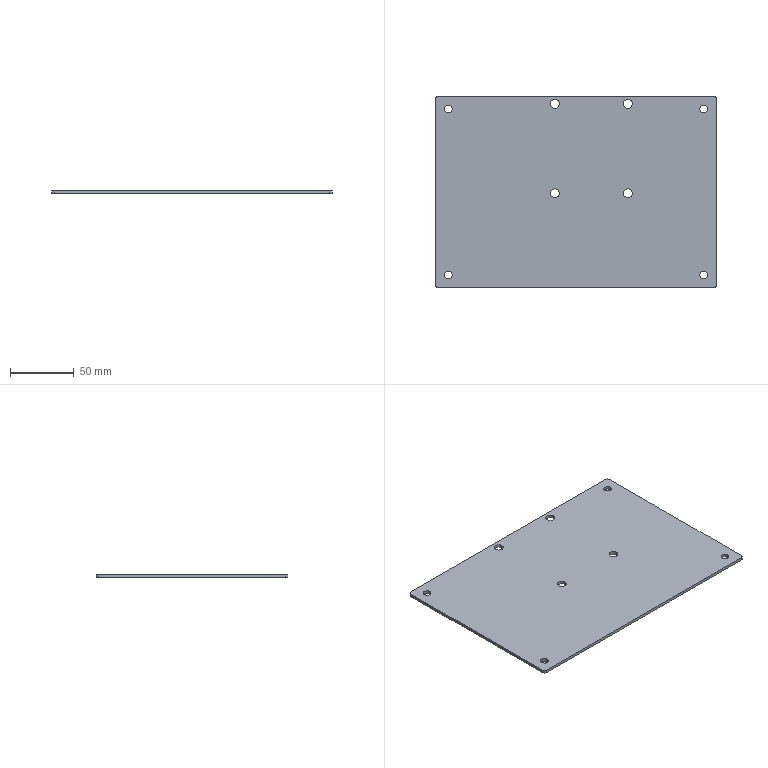Part | STEP file | Second M80U005006A Air System BKT Default | 1 solid | 26 faces | box 220 x 150 x 2.3 mm | volume 75278 mm3 | cylinder 20 | plane 6 | commonest cylinder face diameters 6 x8 7 x8 4 x4
STEP:
#1=CARTESIAN_POINT('',(-20.,69.,0.));
#2=VERTEX_POINT('',#1);
#3=CARTESIAN_POINT('',(-13.,69.,0.));
#4=VERTEX_POINT('',#3);
#5=CARTESIAN_POINT('',(-16.5,69.,0.));
#6=DIRECTION('',(0.,0.,1.));
#7=DIRECTION('',(1.,0.,0.));
#8=AXIS2_PLACEMENT_3D('',#5,#6,#7);
#9=CIRCLE('',#8,3.5);
#10=EDGE_CURVE('',#2,#4,#9,.T.);
#11=ORIENTED_EDGE('',*,*,#10,.F.);
#12=CARTESIAN_POINT('',(-20.,69.,2.3));
#13=VERTEX_POINT('',#12);
#14=CARTESIAN_POINT('',(-20.,69.,2.3));
#15=DIRECTION('',(0.,0.,1.));
#16=VECTOR('',#15,1000.);
#17=LINE('',#14,#16);
#18=EDGE_CURVE('',#2,#13,#17,.T.);
#19=ORIENTED_EDGE('',*,*,#18,.T.);
#20=CARTESIAN_POINT('',(-13.,69.,2.3));
#21=VERTEX_POINT('',#20);
#22=CARTESIAN_POINT('',(-16.5,69.,2.3));
#23=DIRECTION('',(0.,0.,1.));
#24=DIRECTION('',(1.,0.,0.));
#25=AXIS2_PLACEMENT_3D('',#22,#23,#24);
#26=CIRCLE('',#25,3.5);
#27=EDGE_CURVE('',#13,#21,#26,.T.);
#28=ORIENTED_EDGE('',*,*,#27,.T.);
#29=CARTESIAN_POINT('',(-13.,69.,2.3));
#30=DIRECTION('',(0.,0.,1.));
#31=VECTOR('',#30,1000.);
#32=LINE('',#29,#31);
#33=EDGE_CURVE('',#4,#21,#32,.T.);
#34=ORIENTED_EDGE('',*,*,#33,.F.);
#35=EDGE_LOOP('',(#11,#19,#28,#34));
#36=FACE_OUTER_BOUND('',#35,.T.);
#37=CARTESIAN_POINT('',(-16.5,69.,2.3));
#38=DIRECTION('',(0.,0.,1.));
#39=DIRECTION('',(1.,0.,0.));
#40=AXIS2_PLACEMENT_3D('',#37,#38,#39);
#41=CYLINDRICAL_SURFACE('',#40,3.5);
#42=ADVANCED_FACE('',(#36),#41,.F.);
#43=CARTESIAN_POINT('',(37.,69.,0.));
#44=VERTEX_POINT('',#43);
#45=CARTESIAN_POINT('',(44.,69.,0.));
#46=VERTEX_POINT('',#45);
#47=CARTESIAN_POINT('',(40.5,69.,0.));
#48=DIRECTION('',(0.,0.,1.));
#49=DIRECTION('',(1.,0.,0.));
#50=AXIS2_PLACEMENT_3D('',#47,#48,#49);
#51=CIRCLE('',#50,3.5);
#52=EDGE_CURVE('',#44,#46,#51,.T.);
#53=ORIENTED_EDGE('',*,*,#52,.F.);
#54=CARTESIAN_POINT('',(37.,69.,2.3));
#55=VERTEX_POINT('',#54);
#56=CARTESIAN_POINT('',(37.,69.,2.3));
#57=DIRECTION('',(0.,0.,1.));
#58=VECTOR('',#57,1000.);
#59=LINE('',#56,#58);
#60=EDGE_CURVE('',#44,#55,#59,.T.);
#61=ORIENTED_EDGE('',*,*,#60,.T.);
#62=CARTESIAN_POINT('',(44.,69.,2.3));
#63=VERTEX_POINT('',#62);
#64=CARTESIAN_POINT('',(40.5,69.,2.3));
#65=DIRECTION('',(0.,0.,1.));
#66=DIRECTION('',(1.,0.,0.));
#67=AXIS2_PLACEMENT_3D('',#64,#65,#66);
#68=CIRCLE('',#67,3.5);
#69=EDGE_CURVE('',#55,#63,#68,.T.);
#70=ORIENTED_EDGE('',*,*,#69,.T.);
#71=CARTESIAN_POINT('',(44.,69.,2.3));
#72=DIRECTION('',(0.,0.,1.));
#73=VECTOR('',#72,1000.);
#74=LINE('',#71,#73);
#75=EDGE_CURVE('',#46,#63,#74,.T.);
#76=ORIENTED_EDGE('',*,*,#75,.F.);
#77=EDGE_LOOP('',(#53,#61,#70,#76));
#78=FACE_OUTER_BOUND('',#77,.T.);
#79=CARTESIAN_POINT('',(40.5,69.,2.3));
#80=DIRECTION('',(0.,0.,1.));
#81=DIRECTION('',(1.,0.,0.));
#82=AXIS2_PLACEMENT_3D('',#79,#80,#81);
#83=CYLINDRICAL_SURFACE('',#82,3.5);
#84=ADVANCED_FACE('',(#78),#83,.F.);
#85=CARTESIAN_POINT('',(37.,-1.,0.));
#86=VERTEX_POINT('',#85);
#87=CARTESIAN_POINT('',(44.,-1.,0.));
#88=VERTEX_POINT('',#87);
#89=CARTESIAN_POINT('',(40.5,-1.,0.));
#90=DIRECTION('',(0.,0.,1.));
#91=DIRECTION('',(1.,0.,0.));
#92=AXIS2_PLACEMENT_3D('',#89,#90,#91);
#93=CIRCLE('',#92,3.5);
#94=EDGE_CURVE('',#86,#88,#93,.T.);
#95=ORIENTED_EDGE('',*,*,#94,.F.);
#96=CARTESIAN_POINT('',(37.,-1.,2.3));
#97=VERTEX_POINT('',#96);
#98=CARTESIAN_POINT('',(37.,-1.,2.3));
#99=DIRECTION('',(0.,0.,1.));
#100=VECTOR('',#99,1000.);
#101=LINE('',#98,#100);
#102=EDGE_CURVE('',#86,#97,#101,.T.);
#103=ORIENTED_EDGE('',*,*,#102,.T.);
#104=CARTESIAN_POINT('',(44.,-1.,2.3));
#105=VERTEX_POINT('',#104);
#106=CARTESIAN_POINT('',(40.5,-1.,2.3));
#107=DIRECTION('',(0.,0.,1.));
#108=DIRECTION('',(1.,0.,0.));
#109=AXIS2_PLACEMENT_3D('',#106,#107,#108);
#110=CIRCLE('',#109,3.5);
#111=EDGE_CURVE('',#97,#105,#110,.T.);
#112=ORIENTED_EDGE('',*,*,#111,.T.);
#113=CARTESIAN_POINT('',(44.,-1.,2.3));
#114=DIRECTION('',(0.,0.,1.));
#115=VECTOR('',#114,1000.);
#116=LINE('',#113,#115);
#117=EDGE_CURVE('',#88,#105,#116,.T.);
#118=ORIENTED_EDGE('',*,*,#117,.F.);
#119=EDGE_LOOP('',(#95,#103,#112,#118));
#120=FACE_OUTER_BOUND('',#119,.T.);
#121=CARTESIAN_POINT('',(40.5,-1.,2.3));
#122=DIRECTION('',(0.,0.,1.));
#123=DIRECTION('',(1.,0.,0.));
#124=AXIS2_PLACEMENT_3D('',#121,#122,#123);
#125=CYLINDRICAL_SURFACE('',#124,3.5);
#126=ADVANCED_FACE('',(#120),#125,.F.);
#127=CARTESIAN_POINT('',(-20.,-1.,0.));
#128=VERTEX_POINT('',#127);
#129=CARTESIAN_POINT('',(-13.,-1.,0.));
#130=VERTEX_POINT('',#129);
#131=CARTESIAN_POINT('',(-16.5,-1.,0.));
#132=DIRECTION('',(0.,0.,1.));
#133=DIRECTION('',(1.,0.,0.));
#134=AXIS2_PLACEMENT_3D('',#131,#132,#133);
#135=CIRCLE('',#134,3.5);
#136=EDGE_CURVE('',#128,#130,#135,.T.);
#137=ORIENTED_EDGE('',*,*,#136,.F.);
#138=CARTESIAN_POINT('',(-20.,-1.,2.3));
#139=VERTEX_POINT('',#138);
#140=CARTESIAN_POINT('',(-20.,-1.,2.3));
#141=DIRECTION('',(0.,0.,1.));
#142=VECTOR('',#141,1000.);
#143=LINE('',#140,#142);
#144=EDGE_CURVE('',#128,#139,#143,.T.);
#145=ORIENTED_EDGE('',*,*,#144,.T.);
#146=CARTESIAN_POINT('',(-13.,-1.,2.3));
#147=VERTEX_POINT('',#146);
#148=CARTESIAN_POINT('',(-16.5,-1.,2.3));
#149=DIRECTION('',(0.,0.,1.));
#150=DIRECTION('',(1.,0.,0.));
#151=AXIS2_PLACEMENT_3D('',#148,#149,#150);
#152=CIRCLE('',#151,3.5);
#153=EDGE_CURVE('',#139,#147,#152,.T.);
#154=ORIENTED_EDGE('',*,*,#153,.T.);
#155=CARTESIAN_POINT('',(-13.,-1.,2.3));
#156=DIRECTION('',(0.,0.,1.));
#157=VECTOR('',#156,1000.);
#158=LINE('',#155,#157);
#159=EDGE_CURVE('',#130,#147,#158,.T.);
#160=ORIENTED_EDGE('',*,*,#159,.F.);
#161=EDGE_LOOP('',(#137,#145,#154,#160));
#162=FACE_OUTER_BOUND('',#161,.T.);
#163=CARTESIAN_POINT('',(-16.5,-1.,2.3));
#164=DIRECTION('',(0.,0.,1.));
#165=DIRECTION('',(1.,0.,0.));
#166=AXIS2_PLACEMENT_3D('',#163,#164,#165);
#167=CYLINDRICAL_SURFACE('',#166,3.5);
#168=ADVANCED_FACE('',(#162),#167,.F.);
#169=CARTESIAN_POINT('',(-103.,65.,0.));
#170=VERTEX_POINT('',#169);
#171=CARTESIAN_POINT('',(-97.,65.,0.));
#172=VERTEX_POINT('',#171);
#173=CARTESIAN_POINT('',(-100.,65.,0.));
#174=DIRECTION('',(0.,0.,1.));
#175=DIRECTION('',(1.,0.,0.));
#176=AXIS2_PLACEMENT_3D('',#173,#174,#175);
#177=CIRCLE('',#176,3.);
#178=EDGE_CURVE('',#170,#172,#177,.T.);
#179=ORIENTED_EDGE('',*,*,#178,.F.);
#180=CARTESIAN_POINT('',(-103.,65.,2.3));
#181=VERTEX_POINT('',#180);
#182=CARTESIAN_POINT('',(-103.,65.,2.3));
#183=DIRECTION('',(0.,0.,1.));
#184=VECTOR('',#183,1000.);
#185=LINE('',#182,#184);
#186=EDGE_CURVE('',#170,#181,#185,.T.);
#187=ORIENTED_EDGE('',*,*,#186,.T.);
#188=CARTESIAN_POINT('',(-97.,65.,2.3));
#189=VERTEX_POINT('',#188);
#190=CARTESIAN_POINT('',(-100.,65.,2.3));
#191=DIRECTION('',(0.,0.,1.));
#192=DIRECTION('',(1.,0.,0.));
#193=AXIS2_PLACEMENT_3D('',#190,#191,#192);
#194=CIRCLE('',#193,3.);
#195=EDGE_CURVE('',#181,#189,#194,.T.);
#196=ORIENTED_EDGE('',*,*,#195,.T.);
#197=CARTESIAN_POINT('',(-97.,65.,2.3));
#198=DIRECTION('',(0.,0.,1.));
#199=VECTOR('',#198,1000.);
#200=LINE('',#197,#199);
#201=EDGE_CURVE('',#172,#189,#200,.T.);
#202=ORIENTED_EDGE('',*,*,#201,.F.);
#203=EDGE_LOOP('',(#179,#187,#196,#202));
#204=FACE_OUTER_BOUND('',#203,.T.);
#205=CARTESIAN_POINT('',(-100.,65.,2.3));
#206=DIRECTION('',(0.,0.,1.));
#207=DIRECTION('',(1.,0.,0.));
#208=AXIS2_PLACEMENT_3D('',#205,#206,#207);
#209=CYLINDRICAL_SURFACE('',#208,3.);
#210=ADVANCED_FACE('',(#204),#209,.F.);
#211=CARTESIAN_POINT('',(-103.,-65.,0.));
#212=VERTEX_POINT('',#211);
#213=CARTESIAN_POINT('',(-97.,-65.,0.));
#214=VERTEX_POINT('',#213);
#215=CARTESIAN_POINT('',(-100.,-65.,0.));
#216=DIRECTION('',(0.,0.,1.));
#217=DIRECTION('',(1.,0.,0.));
#218=AXIS2_PLACEMENT_3D('',#215,#216,#217);
#219=CIRCLE('',#218,3.);
#220=EDGE_CURVE('',#212,#214,#219,.T.);
#221=ORIENTED_EDGE('',*,*,#220,.F.);
#222=CARTESIAN_POINT('',(-103.,-65.,2.3));
#223=VERTEX_POINT('',#222);
#224=CARTESIAN_POINT('',(-103.,-65.,2.3));
#225=DIRECTION('',(0.,0.,1.));
#226=VECTOR('',#225,1000.);
#227=LINE('',#224,#226);
#228=EDGE_CURVE('',#212,#223,#227,.T.);
#229=ORIENTED_EDGE('',*,*,#228,.T.);
#230=CARTESIAN_POINT('',(-97.,-65.,2.3));
#231=VERTEX_POINT('',#230);
#232=CARTESIAN_POINT('',(-100.,-65.,2.3));
#233=DIRECTION('',(0.,0.,1.));
#234=DIRECTION('',(1.,0.,0.));
#235=AXIS2_PLACEMENT_3D('',#232,#233,#234);
#236=CIRCLE('',#235,3.);
#237=EDGE_CURVE('',#223,#231,#236,.T.);
#238=ORIENTED_EDGE('',*,*,#237,.T.);
#239=CARTESIAN_POINT('',(-97.,-65.,2.3));
#240=DIRECTION('',(0.,0.,1.));
#241=VECTOR('',#240,1000.);
#242=LINE('',#239,#241);
#243=EDGE_CURVE('',#214,#231,#242,.T.);
#244=ORIENTED_EDGE('',*,*,#243,.F.);
#245=EDGE_LOOP('',(#221,#229,#238,#244));
#246=FACE_OUTER_BOUND('',#245,.T.);
#247=CARTESIAN_POINT('',(-100.,-65.,2.3));
#248=DIRECTION('',(0.,0.,1.));
#249=DIRECTION('',(1.,0.,0.));
#250=AXIS2_PLACEMENT_3D('',#247,#248,#249);
#251=CYLINDRICAL_SURFACE('',#250,3.);
#252=ADVANCED_FACE('',(#246),#251,.F.);
#253=CARTESIAN_POINT('',(97.,-65.,0.));
#254=VERTEX_POINT('',#253);
#255=CARTESIAN_POINT('',(103.,-65.,0.));
#256=VERTEX_POINT('',#255);
#257=CARTESIAN_POINT('',(100.,-65.,0.));
#258=DIRECTION('',(0.,0.,1.));
#259=DIRECTION('',(1.,0.,0.));
#260=AXIS2_PLACEMENT_3D('',#257,#258,#259);
#261=CIRCLE('',#260,3.);
#262=EDGE_CURVE('',#254,#256,#261,.T.);
#263=ORIENTED_EDGE('',*,*,#262,.F.);
#264=CARTESIAN_POINT('',(97.,-65.,2.3));
#265=VERTEX_POINT('',#264);
#266=CARTESIAN_POINT('',(97.,-65.,2.3));
#267=DIRECTION('',(0.,0.,1.));
#268=VECTOR('',#267,1000.);
#269=LINE('',#266,#268);
#270=EDGE_CURVE('',#254,#265,#269,.T.);
#271=ORIENTED_EDGE('',*,*,#270,.T.);
#272=CARTESIAN_POINT('',(103.,-65.,2.3));
#273=VERTEX_POINT('',#272);
#274=CARTESIAN_POINT('',(100.,-65.,2.3));
#275=DIRECTION('',(0.,0.,1.));
#276=DIRECTION('',(1.,0.,0.));
#277=AXIS2_PLACEMENT_3D('',#274,#275,#276);
#278=CIRCLE('',#277,3.);
#279=EDGE_CURVE('',#265,#273,#278,.T.);
#280=ORIENTED_EDGE('',*,*,#279,.T.);
#281=CARTESIAN_POINT('',(103.,-65.,2.3));
#282=DIRECTION('',(0.,0.,1.));
#283=VECTOR('',#282,1000.);
#284=LINE('',#281,#283);
#285=EDGE_CURVE('',#256,#273,#284,.T.);
#286=ORIENTED_EDGE('',*,*,#285,.F.);
#287=EDGE_LOOP('',(#263,#271,#280,#286));
#288=FACE_OUTER_BOUND('',#287,.T.);
#289=CARTESIAN_POINT('',(100.,-65.,2.3));
#290=DIRECTION('',(0.,0.,1.));
#291=DIRECTION('',(1.,0.,0.));
#292=AXIS2_PLACEMENT_3D('',#289,#290,#291);
#293=CYLINDRICAL_SURFACE('',#292,3.);
#294=ADVANCED_FACE('',(#288),#293,.F.);
#295=CARTESIAN_POINT('',(97.,65.,0.));
#296=VERTEX_POINT('',#295);
#297=CARTESIAN_POINT('',(103.,65.,0.));
#298=VERTEX_POINT('',#297);
#299=CARTESIAN_POINT('',(100.,65.,0.));
#300=DIRECTION('',(0.,0.,1.));
#301=DIRECTION('',(1.,0.,0.));
#302=AXIS2_PLACEMENT_3D('',#299,#300,#301);
#303=CIRCLE('',#302,3.);
#304=EDGE_CURVE('',#296,#298,#303,.T.);
#305=ORIENTED_EDGE('',*,*,#304,.F.);
#306=CARTESIAN_POINT('',(97.,65.,2.3));
#307=VERTEX_POINT('',#306);
#308=CARTESIAN_POINT('',(97.,65.,2.3));
#309=DIRECTION('',(0.,0.,1.));
#310=VECTOR('',#309,1000.);
#311=LINE('',#308,#310);
#312=EDGE_CURVE('',#296,#307,#311,.T.);
#313=ORIENTED_EDGE('',*,*,#312,.T.);
#314=CARTESIAN_POINT('',(103.,65.,2.3));
#315=VERTEX_POINT('',#314);
#316=CARTESIAN_POINT('',(100.,65.,2.3));
#317=DIRECTION('',(0.,0.,1.));
#318=DIRECTION('',(1.,0.,0.));
#319=AXIS2_PLACEMENT_3D('',#316,#317,#318);
#320=CIRCLE('',#319,3.);
#321=EDGE_CURVE('',#307,#315,#320,.T.);
#322=ORIENTED_EDGE('',*,*,#321,.T.);
#323=CARTESIAN_POINT('',(103.,65.,2.3));
#324=DIRECTION('',(0.,0.,1.));
#325=VECTOR('',#324,1000.);
#326=LINE('',#323,#325);
#327=EDGE_CURVE('',#298,#315,#326,.T.);
#328=ORIENTED_EDGE('',*,*,#327,.F.);
#329=EDGE_LOOP('',(#305,#313,#322,#328));
#330=FACE_OUTER_BOUND('',#329,.T.);
#331=CARTESIAN_POINT('',(100.,65.,2.3));
#332=DIRECTION('',(0.,0.,1.));
#333=DIRECTION('',(1.,0.,0.));
#334=AXIS2_PLACEMENT_3D('',#331,#332,#333);
#335=CYLINDRICAL_SURFACE('',#334,3.);
#336=ADVANCED_FACE('',(#330),#335,.F.);
#337=CARTESIAN_POINT('',(-110.,73.,0.));
#338=VERTEX_POINT('',#337);
#339=CARTESIAN_POINT('',(-110.,-73.,0.));
#340=VERTEX_POINT('',#339);
#341=CARTESIAN_POINT('',(-110.,-75.,0.));
#342=DIRECTION('',(0.,-1.,0.));
#343=VECTOR('',#342,1000.);
#344=LINE('',#341,#343);
#345=EDGE_CURVE('',#338,#340,#344,.T.);
#346=ORIENTED_EDGE('',*,*,#345,.T.);
#347=CARTESIAN_POINT('',(-110.,-73.,2.3));
#348=VERTEX_POINT('',#347);
#349=CARTESIAN_POINT('',(-110.,-73.,2.3));
#350=DIRECTION('',(0.,0.,1.));
#351=VECTOR('',#350,1000.);
#352=LINE('',#349,#351);
#353=EDGE_CURVE('',#340,#348,#352,.T.);
#354=ORIENTED_EDGE('',*,*,#353,.T.);
#355=CARTESIAN_POINT('',(-110.,73.,2.3));
#356=VERTEX_POINT('',#355);
#357=CARTESIAN_POINT('',(-110.,-75.,2.3));
#358=DIRECTION('',(0.,-1.,0.));
#359=VECTOR('',#358,1000.);
#360=LINE('',#357,#359);
#361=EDGE_CURVE('',#356,#348,#360,.T.);
#362=ORIENTED_EDGE('',*,*,#361,.F.);
#363=CARTESIAN_POINT('',(-110.,73.,2.3));
#364=DIRECTION('',(0.,0.,-1.));
#365=VECTOR('',#364,1000.);
#366=LINE('',#363,#365);
#367=EDGE_CURVE('',#356,#338,#366,.T.);
#368=ORIENTED_EDGE('',*,*,#367,.T.);
#369=EDGE_LOOP('',(#346,#354,#362,#368));
#370=FACE_OUTER_BOUND('',#369,.T.);
#371=CARTESIAN_POINT('',(-110.,-75.,2.3));
#372=DIRECTION('',(1.,0.,0.));
#373=DIRECTION('',(0.,0.,-1.));
#374=AXIS2_PLACEMENT_3D('',#371,#372,#373);
#375=PLANE('',#374);
#376=ADVANCED_FACE('',(#370),#375,.F.);
#377=CARTESIAN_POINT('',(-108.,-75.,0.));
#378=VERTEX_POINT('',#377);
#379=CARTESIAN_POINT('',(108.,-75.,0.));
#380=VERTEX_POINT('',#379);
#381=CARTESIAN_POINT('',(110.,-75.,0.));
#382=DIRECTION('',(1.,0.,0.));
#383=VECTOR('',#382,1000.);
#384=LINE('',#381,#383);
#385=EDGE_CURVE('',#378,#380,#384,.T.);
#386=ORIENTED_EDGE('',*,*,#385,.T.);
#387=CARTESIAN_POINT('',(108.,-75.,2.3));
#388=VERTEX_POINT('',#387);
#389=CARTESIAN_POINT('',(108.,-75.,2.3));
#390=DIRECTION('',(0.,0.,1.));
#391=VECTOR('',#390,1000.);
#392=LINE('',#389,#391);
#393=EDGE_CURVE('',#380,#388,#392,.T.);
#394=ORIENTED_EDGE('',*,*,#393,.T.);
#395=CARTESIAN_POINT('',(-108.,-75.,2.3));
#396=VERTEX_POINT('',#395);
#397=CARTESIAN_POINT('',(110.,-75.,2.3));
#398=DIRECTION('',(1.,0.,0.));
#399=VECTOR('',#398,1000.);
#400=LINE('',#397,#399);
#401=EDGE_CURVE('',#396,#388,#400,.T.);
#402=ORIENTED_EDGE('',*,*,#401,.F.);
#403=CARTESIAN_POINT('',(-108.,-75.,2.3));
#404=DIRECTION('',(0.,0.,-1.));
#405=VECTOR('',#404,1000.);
#406=LINE('',#403,#405);
#407=EDGE_CURVE('',#396,#378,#406,.T.);
#408=ORIENTED_EDGE('',*,*,#407,.T.);
#409=EDGE_LOOP('',(#386,#394,#402,#408));
#410=FACE_OUTER_BOUND('',#409,.T.);
#411=CARTESIAN_POINT('',(110.,-75.,2.3));
#412=DIRECTION('',(0.,1.,0.));
#413=DIRECTION('',(-1.,0.,0.));
#414=AXIS2_PLACEMENT_3D('',#411,#412,#413);
#415=PLANE('',#414);
#416=ADVANCED_FACE('',(#410),#415,.F.);
#417=CARTESIAN_POINT('',(110.,-73.,0.));
#418=VERTEX_POINT('',#417);
#419=CARTESIAN_POINT('',(110.,73.,0.));
#420=VERTEX_POINT('',#419);
#421=CARTESIAN_POINT('',(110.,-75.,0.));
#422=DIRECTION('',(0.,1.,0.));
#423=VECTOR('',#422,1000.);
#424=LINE('',#421,#423);
#425=EDGE_CURVE('',#418,#420,#424,.T.);
#426=ORIENTED_EDGE('',*,*,#425,.T.);
#427=CARTESIAN_POINT('',(110.,73.,2.3));
#428=VERTEX_POINT('',#427);
#429=CARTESIAN_POINT('',(110.,73.,2.3));
#430=DIRECTION('',(0.,0.,1.));
#431=VECTOR('',#430,1000.);
#432=LINE('',#429,#431);
#433=EDGE_CURVE('',#420,#428,#432,.T.);
#434=ORIENTED_EDGE('',*,*,#433,.T.);
#435=CARTESIAN_POINT('',(110.,-73.,2.3));
#436=VERTEX_POINT('',#435);
#437=CARTESIAN_POINT('',(110.,-75.,2.3));
#438=DIRECTION('',(0.,1.,0.));
#439=VECTOR('',#438,1000.);
#440=LINE('',#437,#439);
#441=EDGE_CURVE('',#436,#428,#440,.T.);
#442=ORIENTED_EDGE('',*,*,#441,.F.);
#443=CARTESIAN_POINT('',(110.,-73.,2.3));
#444=DIRECTION('',(0.,0.,-1.));
#445=VECTOR('',#444,1000.);
#446=LINE('',#443,#445);
#447=EDGE_CURVE('',#436,#418,#446,.T.);
#448=ORIENTED_EDGE('',*,*,#447,.T.);
#449=EDGE_LOOP('',(#426,#434,#442,#448));
#450=FACE_OUTER_BOUND('',#449,.T.);
#451=CARTESIAN_POINT('',(110.,-75.,2.3));
#452=DIRECTION('',(-1.,0.,0.));
#453=DIRECTION('',(0.,0.,1.));
#454=AXIS2_PLACEMENT_3D('',#451,#452,#453);
#455=PLANE('',#454);
#456=ADVANCED_FACE('',(#450),#455,.F.);
#457=CARTESIAN_POINT('',(108.,75.,2.3));
#458=VERTEX_POINT('',#457);
#459=CARTESIAN_POINT('',(-108.,75.,2.3));
#460=VERTEX_POINT('',#459);
#461=CARTESIAN_POINT('',(110.,75.,2.3));
#462=DIRECTION('',(-1.,0.,0.));
#463=VECTOR('',#462,1000.);
#464=LINE('',#461,#463);
#465=EDGE_CURVE('',#458,#460,#464,.T.);
#466=ORIENTED_EDGE('',*,*,#465,.F.);
#467=CARTESIAN_POINT('',(108.,75.,0.));
#468=VERTEX_POINT('',#467);
#469=CARTESIAN_POINT('',(108.,75.,2.3));
#470=DIRECTION('',(0.,0.,-1.));
#471=VECTOR('',#470,1000.);
#472=LINE('',#469,#471);
#473=EDGE_CURVE('',#458,#468,#472,.T.);
#474=ORIENTED_EDGE('',*,*,#473,.T.);
#475=CARTESIAN_POINT('',(-108.,75.,0.));
#476=VERTEX_POINT('',#475);
#477=CARTESIAN_POINT('',(110.,75.,0.));
#478=DIRECTION('',(-1.,0.,0.));
#479=VECTOR('',#478,1000.);
#480=LINE('',#477,#479);
#481=EDGE_CURVE('',#468,#476,#480,.T.);
#482=ORIENTED_EDGE('',*,*,#481,.T.);
#483=CARTESIAN_POINT('',(-108.,75.,2.3));
#484=DIRECTION('',(0.,0.,1.));
#485=VECTOR('',#484,1000.);
#486=LINE('',#483,#485);
#487=EDGE_CURVE('',#476,#460,#486,.T.);
#488=ORIENTED_EDGE('',*,*,#487,.T.);
#489=EDGE_LOOP('',(#466,#474,#482,#488));
#490=FACE_OUTER_BOUND('',#489,.T.);
#491=CARTESIAN_POINT('',(110.,75.,2.3));
#492=DIRECTION('',(0.,-1.,0.));
#493=DIRECTION('',(1.,0.,0.));
#494=AXIS2_PLACEMENT_3D('',#491,#492,#493);
#495=PLANE('',#494);
#496=ADVANCED_FACE('',(#490),#495,.F.);
#497=CARTESIAN_POINT('',(-16.5,69.,2.3));
#498=DIRECTION('',(0.,0.,1.));
#499=DIRECTION('',(1.,0.,0.));
#500=AXIS2_PLACEMENT_3D('',#497,#498,#499);
#501=CIRCLE('',#500,3.5);
#502=EDGE_CURVE('',#21,#13,#501,.T.);
#503=ORIENTED_EDGE('',*,*,#502,.F.);
#504=ORIENTED_EDGE('',*,*,#27,.F.);
#505=EDGE_LOOP('',(#503,#504));
#506=FACE_BOUND('',#505,.T.);
#507=CARTESIAN_POINT('',(40.5,69.,2.3));
#508=DIRECTION('',(0.,0.,1.));
#509=DIRECTION('',(1.,0.,0.));
#510=AXIS2_PLACEMENT_3D('',#507,#508,#509);
#511=CIRCLE('',#510,3.5);
#512=EDGE_CURVE('',#63,#55,#511,.T.);
#513=ORIENTED_EDGE('',*,*,#512,.F.);
#514=ORIENTED_EDGE('',*,*,#69,.F.);
#515=EDGE_LOOP('',(#513,#514));
#516=FACE_BOUND('',#515,.T.);
#517=CARTESIAN_POINT('',(40.5,-1.,2.3));
#518=DIRECTION('',(0.,0.,1.));
#519=DIRECTION('',(1.,0.,0.));
#520=AXIS2_PLACEMENT_3D('',#517,#518,#519);
#521=CIRCLE('',#520,3.5);
#522=EDGE_CURVE('',#105,#97,#521,.T.);
#523=ORIENTED_EDGE('',*,*,#522,.F.);
#524=ORIENTED_EDGE('',*,*,#111,.F.);
#525=EDGE_LOOP('',(#523,#524));
#526=FACE_BOUND('',#525,.T.);
#527=CARTESIAN_POINT('',(-16.5,-1.,2.3));
#528=DIRECTION('',(0.,0.,1.));
#529=DIRECTION('',(1.,0.,0.));
#530=AXIS2_PLACEMENT_3D('',#527,#528,#529);
#531=CIRCLE('',#530,3.5);
#532=EDGE_CURVE('',#147,#139,#531,.T.);
#533=ORIENTED_EDGE('',*,*,#532,.F.);
#534=ORIENTED_EDGE('',*,*,#153,.F.);
#535=EDGE_LOOP('',(#533,#534));
#536=FACE_BOUND('',#535,.T.);
#537=CARTESIAN_POINT('',(-100.,65.,2.3));
#538=DIRECTION('',(0.,0.,1.));
#539=DIRECTION('',(1.,0.,0.));
#540=AXIS2_PLACEMENT_3D('',#537,#538,#539);
#541=CIRCLE('',#540,3.);
#542=EDGE_CURVE('',#189,#181,#541,.T.);
#543=ORIENTED_EDGE('',*,*,#542,.F.);
#544=ORIENTED_EDGE('',*,*,#195,.F.);
#545=EDGE_LOOP('',(#543,#544));
#546=FACE_BOUND('',#545,.T.);
#547=CARTESIAN_POINT('',(-100.,-65.,2.3));
#548=DIRECTION('',(0.,0.,1.));
#549=DIRECTION('',(1.,0.,0.));
#550=AXIS2_PLACEMENT_3D('',#547,#548,#549);
#551=CIRCLE('',#550,3.);
#552=EDGE_CURVE('',#231,#223,#551,.T.);
#553=ORIENTED_EDGE('',*,*,#552,.F.);
#554=ORIENTED_EDGE('',*,*,#237,.F.);
#555=EDGE_LOOP('',(#553,#554));
#556=FACE_BOUND('',#555,.T.);
#557=CARTESIAN_POINT('',(100.,-65.,2.3));
#558=DIRECTION('',(0.,0.,1.));
#559=DIRECTION('',(1.,0.,0.));
#560=AXIS2_PLACEMENT_3D('',#557,#558,#559);
#561=CIRCLE('',#560,3.);
#562=EDGE_CURVE('',#273,#265,#561,.T.);
#563=ORIENTED_EDGE('',*,*,#562,.F.);
#564=ORIENTED_EDGE('',*,*,#279,.F.);
#565=EDGE_LOOP('',(#563,#564));
#566=FACE_BOUND('',#565,.T.);
#567=CARTESIAN_POINT('',(100.,65.,2.3));
#568=DIRECTION('',(0.,0.,1.));
#569=DIRECTION('',(1.,0.,0.));
#570=AXIS2_PLACEMENT_3D('',#567,#568,#569);
#571=CIRCLE('',#570,3.);
#572=EDGE_CURVE('',#315,#307,#571,.T.);
#573=ORIENTED_EDGE('',*,*,#572,.F.);
#574=ORIENTED_EDGE('',*,*,#321,.F.);
#575=EDGE_LOOP('',(#573,#574));
#576=FACE_BOUND('',#575,.T.);
#577=ORIENTED_EDGE('',*,*,#441,.T.);
#578=CARTESIAN_POINT('',(108.,73.,2.3));
#579=DIRECTION('',(0.,0.,1.));
#580=DIRECTION('',(1.,0.,0.));
#581=AXIS2_PLACEMENT_3D('',#578,#579,#580);
#582=CIRCLE('',#581,2.);
#583=EDGE_CURVE('',#428,#458,#582,.T.);
#584=ORIENTED_EDGE('',*,*,#583,.T.);
#585=ORIENTED_EDGE('',*,*,#465,.T.);
#586=CARTESIAN_POINT('',(-108.,73.,2.3));
#587=DIRECTION('',(0.,0.,1.));
#588=DIRECTION('',(1.,0.,0.));
#589=AXIS2_PLACEMENT_3D('',#586,#587,#588);
#590=CIRCLE('',#589,2.);
#591=EDGE_CURVE('',#460,#356,#590,.T.);
#592=ORIENTED_EDGE('',*,*,#591,.T.);
#593=ORIENTED_EDGE('',*,*,#361,.T.);
#594=CARTESIAN_POINT('',(-108.,-73.,2.3));
#595=DIRECTION('',(0.,0.,1.));
#596=DIRECTION('',(1.,0.,0.));
#597=AXIS2_PLACEMENT_3D('',#594,#595,#596);
#598=CIRCLE('',#597,2.);
#599=EDGE_CURVE('',#348,#396,#598,.T.);
#600=ORIENTED_EDGE('',*,*,#599,.T.);
#601=ORIENTED_EDGE('',*,*,#401,.T.);
#602=CARTESIAN_POINT('',(108.,-73.,2.3));
#603=DIRECTION('',(0.,0.,1.));
#604=DIRECTION('',(1.,0.,0.));
#605=AXIS2_PLACEMENT_3D('',#602,#603,#604);
#606=CIRCLE('',#605,2.);
#607=EDGE_CURVE('',#388,#436,#606,.T.);
#608=ORIENTED_EDGE('',*,*,#607,.T.);
#609=EDGE_LOOP('',(#577,#584,#585,#592,#593,#600,#601,#608));
#610=FACE_OUTER_BOUND('',#609,.T.);
#611=CARTESIAN_POINT('',(0.,0.,2.3));
#612=DIRECTION('',(0.,0.,1.));
#613=DIRECTION('',(1.,0.,0.));
#614=AXIS2_PLACEMENT_3D('',#611,#612,#613);
#615=PLANE('',#614);
#616=ADVANCED_FACE('',(#506,#516,#526,#536,#546,#556,#566,#576,#610),#615,.T.);
#617=CARTESIAN_POINT('',(-16.5,69.,0.));
#618=DIRECTION('',(0.,0.,1.));
#619=DIRECTION('',(1.,0.,0.));
#620=AXIS2_PLACEMENT_3D('',#617,#618,#619);
#621=CIRCLE('',#620,3.5);
#622=EDGE_CURVE('',#4,#2,#621,.T.);
#623=ORIENTED_EDGE('',*,*,#622,.T.);
#624=ORIENTED_EDGE('',*,*,#10,.T.);
#625=EDGE_LOOP('',(#623,#624));
#626=FACE_BOUND('',#625,.T.);
#627=CARTESIAN_POINT('',(40.5,69.,0.));
#628=DIRECTION('',(0.,0.,1.));
#629=DIRECTION('',(1.,0.,0.));
#630=AXIS2_PLACEMENT_3D('',#627,#628,#629);
#631=CIRCLE('',#630,3.5);
#632=EDGE_CURVE('',#46,#44,#631,.T.);
#633=ORIENTED_EDGE('',*,*,#632,.T.);
#634=ORIENTED_EDGE('',*,*,#52,.T.);
#635=EDGE_LOOP('',(#633,#634));
#636=FACE_BOUND('',#635,.T.);
#637=CARTESIAN_POINT('',(40.5,-1.,0.));
#638=DIRECTION('',(0.,0.,1.));
#639=DIRECTION('',(1.,0.,0.));
#640=AXIS2_PLACEMENT_3D('',#637,#638,#639);
#641=CIRCLE('',#640,3.5);
#642=EDGE_CURVE('',#88,#86,#641,.T.);
#643=ORIENTED_EDGE('',*,*,#642,.T.);
#644=ORIENTED_EDGE('',*,*,#94,.T.);
#645=EDGE_LOOP('',(#643,#644));
#646=FACE_BOUND('',#645,.T.);
#647=CARTESIAN_POINT('',(-16.5,-1.,0.));
#648=DIRECTION('',(0.,0.,1.));
#649=DIRECTION('',(1.,0.,0.));
#650=AXIS2_PLACEMENT_3D('',#647,#648,#649);
#651=CIRCLE('',#650,3.5);
#652=EDGE_CURVE('',#130,#128,#651,.T.);
#653=ORIENTED_EDGE('',*,*,#652,.T.);
#654=ORIENTED_EDGE('',*,*,#136,.T.);
#655=EDGE_LOOP('',(#653,#654));
#656=FACE_BOUND('',#655,.T.);
#657=CARTESIAN_POINT('',(-100.,65.,0.));
#658=DIRECTION('',(0.,0.,1.));
#659=DIRECTION('',(1.,0.,0.));
#660=AXIS2_PLACEMENT_3D('',#657,#658,#659);
#661=CIRCLE('',#660,3.);
#662=EDGE_CURVE('',#172,#170,#661,.T.);
#663=ORIENTED_EDGE('',*,*,#662,.T.);
#664=ORIENTED_EDGE('',*,*,#178,.T.);
#665=EDGE_LOOP('',(#663,#664));
#666=FACE_BOUND('',#665,.T.);
#667=CARTESIAN_POINT('',(-100.,-65.,0.));
#668=DIRECTION('',(0.,0.,1.));
#669=DIRECTION('',(1.,0.,0.));
#670=AXIS2_PLACEMENT_3D('',#667,#668,#669);
#671=CIRCLE('',#670,3.);
#672=EDGE_CURVE('',#214,#212,#671,.T.);
#673=ORIENTED_EDGE('',*,*,#672,.T.);
#674=ORIENTED_EDGE('',*,*,#220,.T.);
#675=EDGE_LOOP('',(#673,#674));
#676=FACE_BOUND('',#675,.T.);
#677=CARTESIAN_POINT('',(100.,-65.,0.));
#678=DIRECTION('',(0.,0.,1.));
#679=DIRECTION('',(1.,0.,0.));
#680=AXIS2_PLACEMENT_3D('',#677,#678,#679);
#681=CIRCLE('',#680,3.);
#682=EDGE_CURVE('',#256,#254,#681,.T.);
#683=ORIENTED_EDGE('',*,*,#682,.T.);
#684=ORIENTED_EDGE('',*,*,#262,.T.);
#685=EDGE_LOOP('',(#683,#684));
#686=FACE_BOUND('',#685,.T.);
#687=CARTESIAN_POINT('',(100.,65.,0.));
#688=DIRECTION('',(0.,0.,1.));
#689=DIRECTION('',(1.,0.,0.));
#690=AXIS2_PLACEMENT_3D('',#687,#688,#689);
#691=CIRCLE('',#690,3.);
#692=EDGE_CURVE('',#298,#296,#691,.T.);
#693=ORIENTED_EDGE('',*,*,#692,.T.);
#694=ORIENTED_EDGE('',*,*,#304,.T.);
#695=EDGE_LOOP('',(#693,#694));
#696=FACE_BOUND('',#695,.T.);
#697=ORIENTED_EDGE('',*,*,#481,.F.);
#698=CARTESIAN_POINT('',(108.,73.,0.));
#699=DIRECTION('',(0.,0.,-1.));
#700=DIRECTION('',(1.,0.,0.));
#701=AXIS2_PLACEMENT_3D('',#698,#699,#700);
#702=CIRCLE('',#701,2.);
#703=EDGE_CURVE('',#468,#420,#702,.T.);
#704=ORIENTED_EDGE('',*,*,#703,.T.);
#705=ORIENTED_EDGE('',*,*,#425,.F.);
#706=CARTESIAN_POINT('',(108.,-73.,0.));
#707=DIRECTION('',(0.,0.,-1.));
#708=DIRECTION('',(1.,0.,0.));
#709=AXIS2_PLACEMENT_3D('',#706,#707,#708);
#710=CIRCLE('',#709,2.);
#711=EDGE_CURVE('',#418,#380,#710,.T.);
#712=ORIENTED_EDGE('',*,*,#711,.T.);
#713=ORIENTED_EDGE('',*,*,#385,.F.);
#714=CARTESIAN_POINT('',(-108.,-73.,0.));
#715=DIRECTION('',(0.,0.,-1.));
#716=DIRECTION('',(1.,0.,0.));
#717=AXIS2_PLACEMENT_3D('',#714,#715,#716);
#718=CIRCLE('',#717,2.);
#719=EDGE_CURVE('',#378,#340,#718,.T.);
#720=ORIENTED_EDGE('',*,*,#719,.T.);
#721=ORIENTED_EDGE('',*,*,#345,.F.);
#722=CARTESIAN_POINT('',(-108.,73.,0.));
#723=DIRECTION('',(0.,0.,-1.));
#724=DIRECTION('',(1.,0.,0.));
#725=AXIS2_PLACEMENT_3D('',#722,#723,#724);
#726=CIRCLE('',#725,2.);
#727=EDGE_CURVE('',#338,#476,#726,.T.);
#728=ORIENTED_EDGE('',*,*,#727,.T.);
#729=EDGE_LOOP('',(#697,#704,#705,#712,#713,#720,#721,#728));
#730=FACE_OUTER_BOUND('',#729,.T.);
#731=CARTESIAN_POINT('',(0.,0.,0.));
#732=DIRECTION('',(0.,0.,1.));
#733=DIRECTION('',(1.,0.,0.));
#734=AXIS2_PLACEMENT_3D('',#731,#732,#733);
#735=PLANE('',#734);
#736=ADVANCED_FACE('',(#626,#636,#646,#656,#666,#676,#686,#696,#730),#735,.F.);
#737=ORIENTED_EDGE('',*,*,#312,.F.);
#738=ORIENTED_EDGE('',*,*,#692,.F.);
#739=ORIENTED_EDGE('',*,*,#327,.T.);
#740=ORIENTED_EDGE('',*,*,#572,.T.);
#741=EDGE_LOOP('',(#737,#738,#739,#740));
#742=FACE_OUTER_BOUND('',#741,.T.);
#743=CARTESIAN_POINT('',(100.,65.,2.3));
#744=DIRECTION('',(0.,0.,1.));
#745=DIRECTION('',(1.,0.,0.));
#746=AXIS2_PLACEMENT_3D('',#743,#744,#745);
#747=CYLINDRICAL_SURFACE('',#746,3.);
#748=ADVANCED_FACE('',(#742),#747,.F.);
#749=ORIENTED_EDGE('',*,*,#270,.F.);
#750=ORIENTED_EDGE('',*,*,#682,.F.);
#751=ORIENTED_EDGE('',*,*,#285,.T.);
#752=ORIENTED_EDGE('',*,*,#562,.T.);
#753=EDGE_LOOP('',(#749,#750,#751,#752));
#754=FACE_OUTER_BOUND('',#753,.T.);
#755=CARTESIAN_POINT('',(100.,-65.,2.3));
#756=DIRECTION('',(0.,0.,1.));
#757=DIRECTION('',(1.,0.,0.));
#758=AXIS2_PLACEMENT_3D('',#755,#756,#757);
#759=CYLINDRICAL_SURFACE('',#758,3.);
#760=ADVANCED_FACE('',(#754),#759,.F.);
#761=ORIENTED_EDGE('',*,*,#228,.F.);
#762=ORIENTED_EDGE('',*,*,#672,.F.);
#763=ORIENTED_EDGE('',*,*,#243,.T.);
#764=ORIENTED_EDGE('',*,*,#552,.T.);
#765=EDGE_LOOP('',(#761,#762,#763,#764));
#766=FACE_OUTER_BOUND('',#765,.T.);
#767=CARTESIAN_POINT('',(-100.,-65.,2.3));
#768=DIRECTION('',(0.,0.,1.));
#769=DIRECTION('',(1.,0.,0.));
#770=AXIS2_PLACEMENT_3D('',#767,#768,#769);
#771=CYLINDRICAL_SURFACE('',#770,3.);
#772=ADVANCED_FACE('',(#766),#771,.F.);
#773=ORIENTED_EDGE('',*,*,#186,.F.);
#774=ORIENTED_EDGE('',*,*,#662,.F.);
#775=ORIENTED_EDGE('',*,*,#201,.T.);
#776=ORIENTED_EDGE('',*,*,#542,.T.);
#777=EDGE_LOOP('',(#773,#774,#775,#776));
#778=FACE_OUTER_BOUND('',#777,.T.);
#779=CARTESIAN_POINT('',(-100.,65.,2.3));
#780=DIRECTION('',(0.,0.,1.));
#781=DIRECTION('',(1.,0.,0.));
#782=AXIS2_PLACEMENT_3D('',#779,#780,#781);
#783=CYLINDRICAL_SURFACE('',#782,3.);
#784=ADVANCED_FACE('',(#778),#783,.F.);
#785=ORIENTED_EDGE('',*,*,#144,.F.);
#786=ORIENTED_EDGE('',*,*,#652,.F.);
#787=ORIENTED_EDGE('',*,*,#159,.T.);
#788=ORIENTED_EDGE('',*,*,#532,.T.);
#789=EDGE_LOOP('',(#785,#786,#787,#788));
#790=FACE_OUTER_BOUND('',#789,.T.);
#791=CARTESIAN_POINT('',(-16.5,-1.,2.3));
#792=DIRECTION('',(0.,0.,1.));
#793=DIRECTION('',(1.,0.,0.));
#794=AXIS2_PLACEMENT_3D('',#791,#792,#793);
#795=CYLINDRICAL_SURFACE('',#794,3.5);
#796=ADVANCED_FACE('',(#790),#795,.F.);
#797=ORIENTED_EDGE('',*,*,#102,.F.);
#798=ORIENTED_EDGE('',*,*,#642,.F.);
#799=ORIENTED_EDGE('',*,*,#117,.T.);
#800=ORIENTED_EDGE('',*,*,#522,.T.);
#801=EDGE_LOOP('',(#797,#798,#799,#800));
#802=FACE_OUTER_BOUND('',#801,.T.);
#803=CARTESIAN_POINT('',(40.5,-1.,2.3));
#804=DIRECTION('',(0.,0.,1.));
#805=DIRECTION('',(1.,0.,0.));
#806=AXIS2_PLACEMENT_3D('',#803,#804,#805);
#807=CYLINDRICAL_SURFACE('',#806,3.5);
#808=ADVANCED_FACE('',(#802),#807,.F.);
#809=ORIENTED_EDGE('',*,*,#60,.F.);
#810=ORIENTED_EDGE('',*,*,#632,.F.);
#811=ORIENTED_EDGE('',*,*,#75,.T.);
#812=ORIENTED_EDGE('',*,*,#512,.T.);
#813=EDGE_LOOP('',(#809,#810,#811,#812));
#814=FACE_OUTER_BOUND('',#813,.T.);
#815=CARTESIAN_POINT('',(40.5,69.,2.3));
#816=DIRECTION('',(0.,0.,1.));
#817=DIRECTION('',(1.,0.,0.));
#818=AXIS2_PLACEMENT_3D('',#815,#816,#817);
#819=CYLINDRICAL_SURFACE('',#818,3.5);
#820=ADVANCED_FACE('',(#814),#819,.F.);
#821=ORIENTED_EDGE('',*,*,#18,.F.);
#822=ORIENTED_EDGE('',*,*,#622,.F.);
#823=ORIENTED_EDGE('',*,*,#33,.T.);
#824=ORIENTED_EDGE('',*,*,#502,.T.);
#825=EDGE_LOOP('',(#821,#822,#823,#824));
#826=FACE_OUTER_BOUND('',#825,.T.);
#827=CARTESIAN_POINT('',(-16.5,69.,2.3));
#828=DIRECTION('',(0.,0.,1.));
#829=DIRECTION('',(1.,0.,0.));
#830=AXIS2_PLACEMENT_3D('',#827,#828,#829);
#831=CYLINDRICAL_SURFACE('',#830,3.5);
#832=ADVANCED_FACE('',(#826),#831,.F.);
#833=ORIENTED_EDGE('',*,*,#583,.F.);
#834=ORIENTED_EDGE('',*,*,#433,.F.);
#835=ORIENTED_EDGE('',*,*,#703,.F.);
#836=ORIENTED_EDGE('',*,*,#473,.F.);
#837=EDGE_LOOP('',(#833,#834,#835,#836));
#838=FACE_OUTER_BOUND('',#837,.T.);
#839=CARTESIAN_POINT('',(108.,73.,2.3));
#840=DIRECTION('',(0.,0.,-1.));
#841=DIRECTION('',(-1.,0.,0.));
#842=AXIS2_PLACEMENT_3D('',#839,#840,#841);
#843=CYLINDRICAL_SURFACE('',#842,2.);
#844=ADVANCED_FACE('',(#838),#843,.T.);
#845=ORIENTED_EDGE('',*,*,#607,.F.);
#846=ORIENTED_EDGE('',*,*,#393,.F.);
#847=ORIENTED_EDGE('',*,*,#711,.F.);
#848=ORIENTED_EDGE('',*,*,#447,.F.);
#849=EDGE_LOOP('',(#845,#846,#847,#848));
#850=FACE_OUTER_BOUND('',#849,.T.);
#851=CARTESIAN_POINT('',(108.,-73.,2.3));
#852=DIRECTION('',(0.,0.,-1.));
#853=DIRECTION('',(-1.,0.,0.));
#854=AXIS2_PLACEMENT_3D('',#851,#852,#853);
#855=CYLINDRICAL_SURFACE('',#854,2.);
#856=ADVANCED_FACE('',(#850),#855,.T.);
#857=ORIENTED_EDGE('',*,*,#599,.F.);
#858=ORIENTED_EDGE('',*,*,#353,.F.);
#859=ORIENTED_EDGE('',*,*,#719,.F.);
#860=ORIENTED_EDGE('',*,*,#407,.F.);
#861=EDGE_LOOP('',(#857,#858,#859,#860));
#862=FACE_OUTER_BOUND('',#861,.T.);
#863=CARTESIAN_POINT('',(-108.,-73.,2.3));
#864=DIRECTION('',(0.,0.,-1.));
#865=DIRECTION('',(-1.,0.,0.));
#866=AXIS2_PLACEMENT_3D('',#863,#864,#865);
#867=CYLINDRICAL_SURFACE('',#866,2.);
#868=ADVANCED_FACE('',(#862),#867,.T.);
#869=ORIENTED_EDGE('',*,*,#591,.F.);
#870=ORIENTED_EDGE('',*,*,#487,.F.);
#871=ORIENTED_EDGE('',*,*,#727,.F.);
#872=ORIENTED_EDGE('',*,*,#367,.F.);
#873=EDGE_LOOP('',(#869,#870,#871,#872));
#874=FACE_OUTER_BOUND('',#873,.T.);
#875=CARTESIAN_POINT('',(-108.,73.,2.3));
#876=DIRECTION('',(0.,0.,-1.));
#877=DIRECTION('',(-1.,0.,0.));
#878=AXIS2_PLACEMENT_3D('',#875,#876,#877);
#879=CYLINDRICAL_SURFACE('',#878,2.);
#880=ADVANCED_FACE('',(#874),#879,.T.);
#881=CLOSED_SHELL('',(#42,#84,#126,#168,#210,#252,#294,#336,#376,#416,#456,#496,#616,#736,#748,#760,#772,#784,#796,#808,#820,#832,#844,#856,#868,#880));
#882=MANIFOLD_SOLID_BREP('',#881);
#883=CARTESIAN_POINT('',(0.,0.,0.));
#884=DIRECTION('',(0.,0.,1.));
#885=DIRECTION('',(1.,0.,0.));
#886=AXIS2_PLACEMENT_3D('',#883,#884,#885);
#887=(LENGTH_UNIT()NAMED_UNIT(*)SI_UNIT(.MILLI.,.METRE.));
#888=UNCERTAINTY_MEASURE_WITH_UNIT(LENGTH_MEASURE(0.00001),#887,'','');
#889=(NAMED_UNIT(*)PLANE_ANGLE_UNIT()SI_UNIT($,.RADIAN.));
#890=(NAMED_UNIT(*)SI_UNIT($,.STERADIAN.)SOLID_ANGLE_UNIT());
#891=(GEOMETRIC_REPRESENTATION_CONTEXT(3)GLOBAL_UNCERTAINTY_ASSIGNED_CONTEXT((#888))GLOBAL_UNIT_ASSIGNED_CONTEXT((#887,#889,#890))REPRESENTATION_CONTEXT('',''));
#892=ADVANCED_BREP_SHAPE_REPRESENTATION('',(#882,#886),#891);